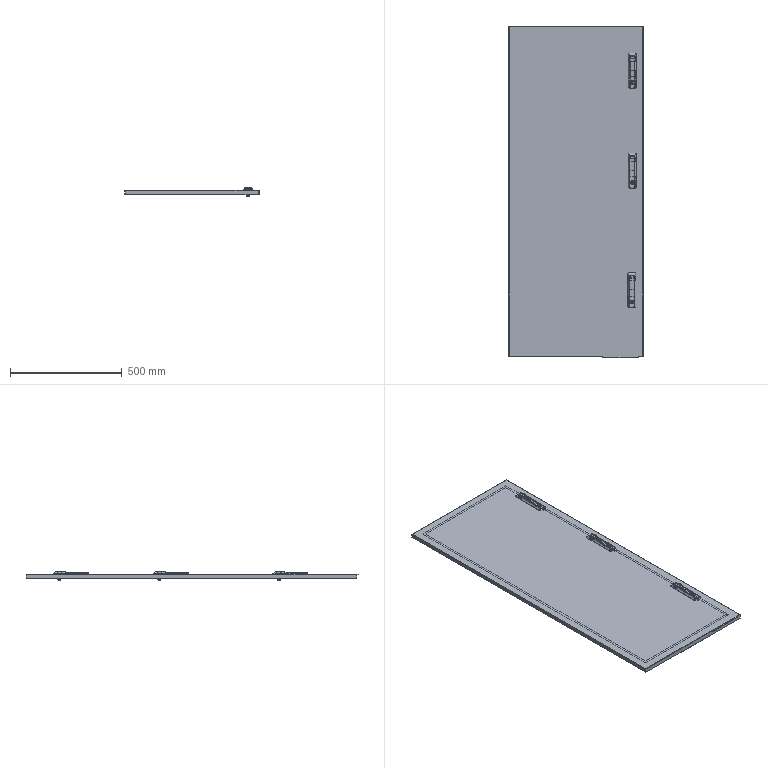Part | SolidWorks | 13 solids | 1927 faces | box 599 x 1482 x 37.95 mm | volume 2644503 mm3 | plane 1328 | cylinder 449 | spline 132 | cone 18 | commonest cylinder face diameters 1 x45 10 x36 1000 x36 8 x30 4 x24 12 x21